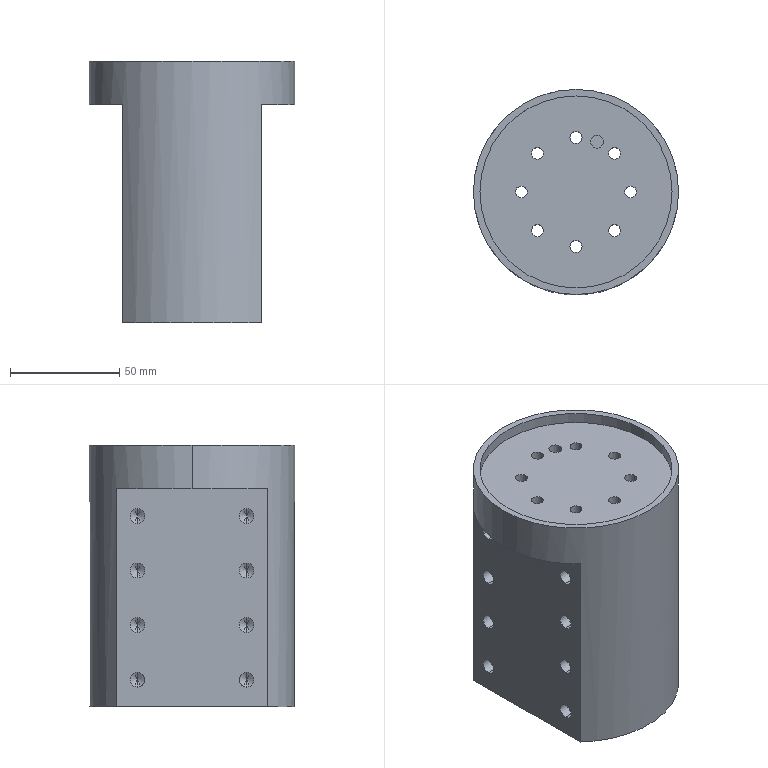Part | NX | features BREP 1 | 1 solid | 94 faces | box 94 x 94 x 120 mm | volume 601070 mm3 | cylinder 54 | cone 32 | plane 8 | commonest cylinder face diameters 5.5 x16 6.8 x16 12 x16 6 x2 88 x2 94 x2